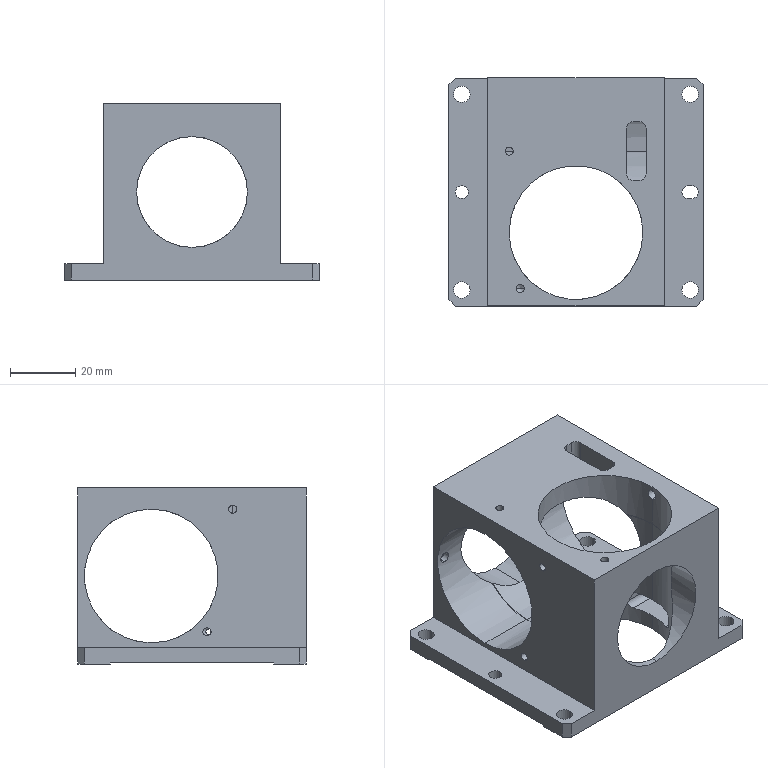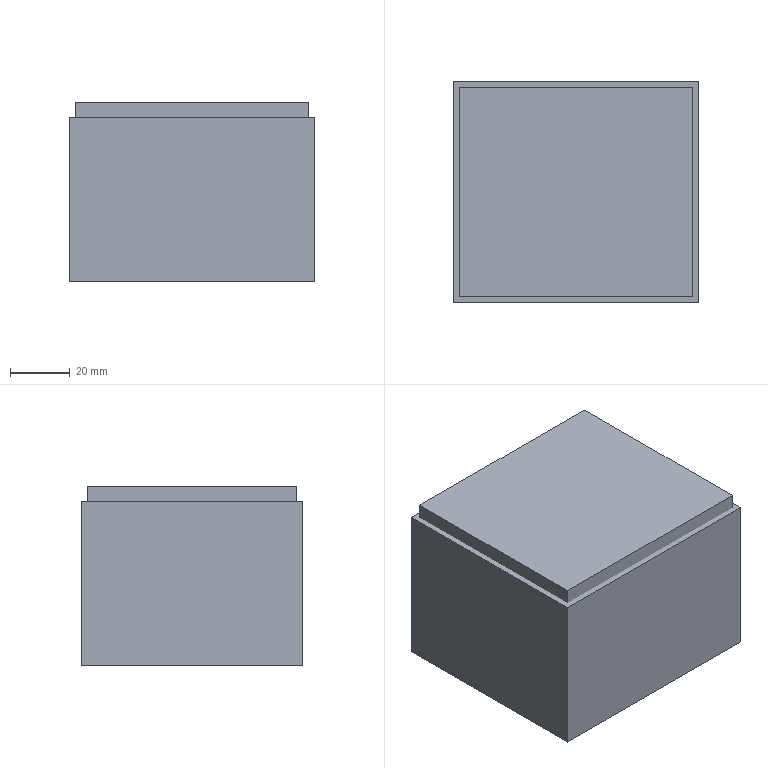CAM job | NX | 3+2 milling, drilling | part box 78 x 70 x 54 mm | stock box 82 x 74 x 60 mm
Tools:
number,name,description,diameter,corner_radius,flute_length,length,flutes
1,D63,Milling Tool-5 Parameters,63.0,0.0,50.0,75.0,2
7,D6A45,Milling Tool-5 Parameters,6.0,0.0,50.0,75.0,2
2,D20,Milling Tool-5 Parameters,20.0,0.0,50.0,75.0,2
13,D16JING,Milling Tool-5 Parameters,16.0,0.0,50.0,75.0,2
4,D4,Milling Tool-5 Parameters,4.0,0.0,50.0,75.0,2
10,D10,Milling Tool-5 Parameters,10.0,0.0,50.0,75.0,2
11,D10JING,Milling Tool-5 Parameters,10.0,0.0,50.0,75.0,2
5,5.0ZT,Drilling Tool,5.0,0.0,35.0,50.0,2
3,D3,Milling Tool-5 Parameters,3.0,0.0,50.0,75.0,2
3,3.3ZT,Drilling Tool,3.3,0.0,35.0,50.0,2
12,2.5ZT,Drilling Tool,2.5,0.0,35.0,50.0,2
Operations:
program,operation,operation_type,tool,method,geometry_group,spindle_rpm,surface_speed,feed_per_tooth,feed_cut,feed_plunge,cut_length_mm,path_length_mm,cut_time_min,machine_time_min
1,FLOOR_WALL,VolumeBased25DMillingOperation,D63,METHOD,A,6500.0,1286.0,0.1154,1500.0,100.0,350.797,404.797,0.2339,0.2393
1,DRILLING,Operation,D6A45,METHOD,A,5000.0,94.0,0.025,250.0,0.0,13.8,150.438,0.0552,0.0689
1,ZLEVEL_PROFILE,ZLevelMilling,D20,METHOD,A,9500.0,298.0,0.1579,3000.0,1000.0,38384.406,38495.406,12.82,12.831
1,FLOOR_WALL_1,VolumeBased25DMillingOperation,D20,METHOD,A,9500.0,298.0,0.1316,2500.0,1000.0,39414.058,40636.117,16.148,16.27
1,HOLE_MILLING,CylinderMilling,D20,METHOD,A,9500.0,596.0,0.1053,2000.0,100.0,7220.845,7334.345,3.61,3.622
1,FLOOR_WALL_1_COPY,VolumeBased25DMillingOperation,D16JING,METHOD,A,9500.0,298.0,0.0632,1200.0,1000.0,547.085,941.006,0.4579,0.4972
1,FLOOR_WALL_1_COPY_COPY,VolumeBased25DMillingOperation,D16JING,METHOD,A,9500.0,298.0,0.0632,1200.0,1000.0,913.468,1960.478,0.7673,0.872
1,CAVITY_MILL_COPY_1,CavityMilling,D16JING,METHOD,A,9500.0,298.0,0.0632,1200.0,1000.0,1363.231,1764.306,1.139,1.179
1,ZLEVEL_PROFILE_1,ZLevelMilling,D4,METHOD,A,9500.0,119.0,0.0658,1250.0,100.0,876.915,943.728,0.7015,0.7082
1,PLANAR_MILL_COPY_1,PlanarMilling,D6A45,METHOD,A,9500.0,179.0,0.0658,1250.0,100.0,427.858,673.736,0.3423,0.3669
1,TOOLCOMP,CylinderMilling,D16JING,METHOD,A,9500.0,477.0,0.0526,1000.0,100.0,537.458,650.958,0.5375,0.5488
2,FLOOR_WALL_COPY,VolumeBased25DMillingOperation,D63,METHOD,B,6500.0,1286.0,0.1154,1500.0,100.0,2056.782,2574.768,1.371,1.423
2,FLOOR_WALL_1_COPY_1,VolumeBased25DMillingOperation,D10,METHOD,B,9500.0,298.0,0.1316,2500.0,1000.0,882.449,943.249,0.3546,0.3607
2,FLOOR_WALL_1_COPY_COPY_1,VolumeBased25DMillingOperation,D10JING,METHOD,B,9500.0,298.0,0.0632,1200.0,1000.0,1079.131,1237.281,0.9015,0.9173
2,DRILLING_1,Operation,D6A45,METHOD,B,5000.0,94.0,0.025,250.0,0.0,16.4,292.014,0.0656,0.0932
2,DRILLING_1_COPY,Operation,5.0ZT,METHOD,B,2000.0,31.0,0.0625,250.0,0.0,44.009,347.231,0.176,0.2064
2,HOLE_MILLING_1,CylinderMilling,D3,METHOD,B,9500.0,89.0,0.0658,1250.0,100.0,87.695,152.695,0.0702,0.0767
2,ZLEVEL_PROFILE_1_1,ZLevelMilling,D3,METHOD,B,9500.0,89.0,0.0789,1500.0,100.0,149.323,223.523,0.0995,0.107
2,PLANAR_MILL_COPY_1_1_COPY,PlanarMilling,D6A45,METHOD,B,9500.0,179.0,0.0658,1250.0,100.0,317.588,898.175,0.2541,0.3121
2,PLANAR_MILL_COPY_1_1_COPY_COPY,PlanarMilling,D6A45,METHOD,B,9500.0,179.0,0.0658,1250.0,100.0,228.549,747.869,0.1828,0.2348
2,TOOLCOMP_1,CylinderMilling,D3,METHOD,B,9500.0,89.0,0.0658,1250.0,100.0,12.884,77.884,0.0103,0.0168
2,TOOLCOMP1,ZLevelMilling,D3,METHOD,B,9500.0,89.0,0.0632,1200.0,100.0,9.842,75.342,0.0082,0.0148
3,HOLE_MILLING_COPY,CylinderMilling,D20,METHOD,C,9500.0,596.0,0.0789,1500.0,100.0,6178.349,6307.849,4.119,4.132
3,11,CylinderMilling,D16JING,METHOD,C,9500.0,477.0,0.0526,1000.0,100.0,483.37,612.87,0.4834,0.4963
3,DRILLING_1_COPY_1,Operation,D6A45,METHOD,C,5000.0,94.0,0.025,250.0,0.0,4.1,68.2,0.0164,0.0228
3,DRILLING_1_COPY_1_COPY,Operation,3.3ZT,METHOD,C,2000.0,20.0,0.0375,150.0,0.0,7.558,75.116,0.0504,0.0571
3,PLANAR_MILL_COPY_1_1_COPY_COPY_1,PlanarMilling,D6A45,METHOD,C,9500.0,179.0,0.0658,1250.0,100.0,120.534,265.018,0.0964,0.1109
4,HOLE_MILLING_COPY_1,CylinderMilling,D20,METHOD,D,9500.0,596.0,0.1053,2000.0,100.0,7220.845,7358.345,3.61,3.624
4,DRILLING_1_COPY_1_COPY_1,Operation,D6A45,METHOD,D,5000.0,94.0,0.025,250.0,0.0,9.0,143.538,0.036,0.0495
4,DRILLING_COPY_COPY,Operation,2.5ZT,METHOD,D,2000.0,15.0,0.03,120.0,0.0,23.04,171.619,0.192,0.2069
4,PLANAR_MILL_COPY_1_1_COPY_COPY_1_COPY,PlanarMilling,D6A45,METHOD,D,9500.0,179.0,0.0658,1250.0,100.0,116.666,199.666,0.0933,0.1016
4,TOOLCOMP_COPY,CylinderMilling,D16JING,METHOD,D,9500.0,477.0,0.0526,1000.0,100.0,537.458,674.958,0.5375,0.5512
5,DRILLING_1_COPY_1_COPY_2,Operation,D6A45,METHOD,E,5000.0,94.0,0.025,250.0,0.0,4.75,93.5,0.019,0.0279
5,DRILLING_1_COPY_1_COPY_COPY,Operation,3.3ZT,METHOD,E,2000.0,20.0,0.0375,150.0,0.0,12.058,108.116,0.0804,0.09
5,ZLEVEL_PROFILE_1_COPY,ZLevelMilling,D4,METHOD,E,9500.0,119.0,0.0658,1250.0,100.0,909.438,1000.867,0.7276,0.7367
5,PLANAR_MILL_COPY_1_1_COPY_COPY_1_COPY_COPY,PlanarMilling,D6A45,METHOD,E,9500.0,179.0,0.0658,1250.0,100.0,157.018,489.722,0.1256,0.1589
5,TOOLCOMP_COPY_COPY,CylinderMilling,D16JING,METHOD,E,9500.0,477.0,0.0526,1000.0,100.0,690.915,810.415,0.6909,0.7029